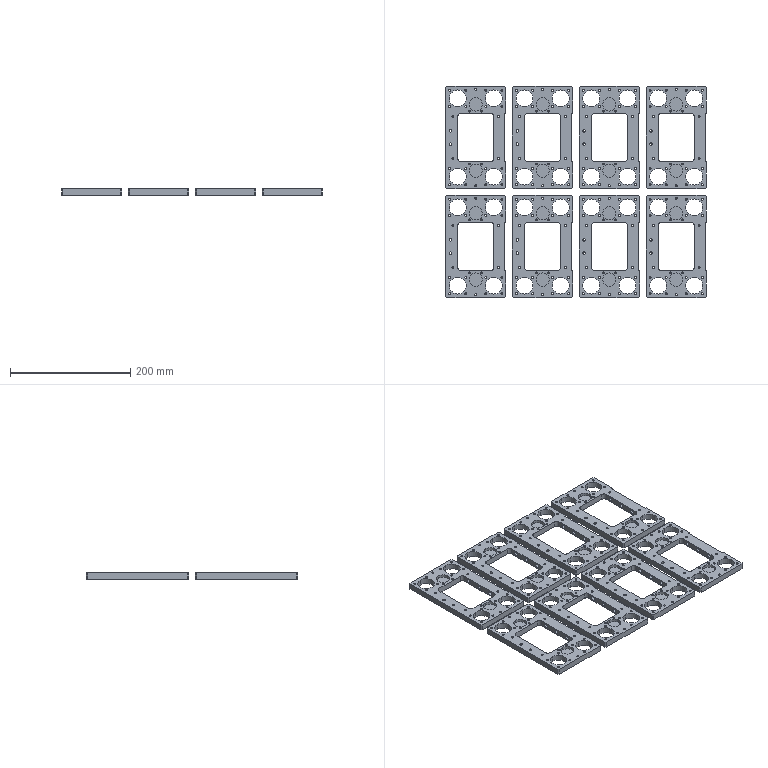NC program | NX | posted with a generic post | part box 433 x 351 x 10 mm
Whole program:
N10 G17 G21 G94 G90
(DRILLING_COPY_1 , TOOL : D6A45)
N12 T01 M6
N14 G54
N16 G17 G0 G90 X25. Y0. B0. C0. S5000 M3
N18 G43 Z30. H1
N20 G94 G81 G98 Z-3. F350. R1.
N22 X0.
N24 X-25.
N26 G80
N28 G0 X-25. Y0. Z30.
N30 M5
(DRILLING_COPY_COPY_COPY , TOOL : 6.5ZT)
N32 T10 M6
N34 G54
N36 G17 G0 G90 X-25. Y0. B0. C0. S2000 M3
N38 G43 Z30. H10
N40 G94 G83 G98 Z-23.453 F300. Q2. R1.
N42 X0.
N44 X25.
N46 G80
N48 G0 X25. Y0. Z30.
N50 M5
(刀补 , TOOL : D6)
N52 T12 M6
N54 G54
N56 G17 G0 G90 X36.894 Y-5.324 B0. C0. S9500 M3
N58 G43 Z30. H12
N60 Z-1.
N62 G94 G1 Z-2. F1000.
N64 G41 X36.95 Y-5.241 D12
N66 G3 X37. Y-5. R0.6
N68 G1 Y5. F1500.
N70 G3 X36.95 Y5.241 R0.6
N72 G40
N74 G1 X36.894 Y5.324
N76 Z-1.
N78 G0 Z30.
N80 X-36.894
N82 Z-1.
N84 G1 Z-2. F1000.
N86 G41 X-36.95 Y5.241
N88 G3 X-37. Y5. R0.6
N90 G1 Y-5. F1500.
N92 G3 X-36.95 Y-5.241 R0.6
N94 G40
N96 G1 X-36.894 Y-5.324
N98 Z-1.
N100 G0 Z30.
N102 M5
N104 M2